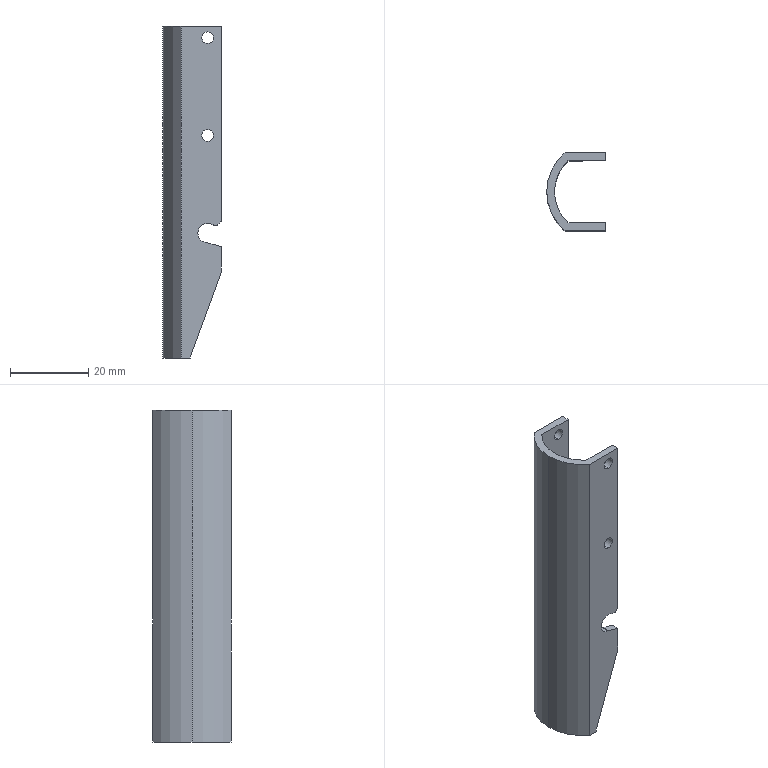Part | SolidWorks | features Fillet 2, ICE 2, Extrusion 1 | 1 solid | 40 faces | box 15 x 20 x 85 mm | volume 6317 mm3 | cylinder 22 | plane 18 | commonest cylinder face diameters 1 x8 3 x8 5 x2 22 x2 26 x2
STEP:
#1=CARTESIAN_POINT('',(-1.5,-8.,83.5));
#2=VERTEX_POINT('',#1);
#3=CARTESIAN_POINT('',(-1.5,-8.,80.5));
#4=VERTEX_POINT('',#3);
#5=CARTESIAN_POINT('',(-1.5,-8.,82.));
#6=DIRECTION('',(0.,-1.,0.));
#7=DIRECTION('',(1.,0.,0.));
#8=AXIS2_PLACEMENT_3D('',#5,#6,#7);
#9=CIRCLE('',#8,1.5);
#10=EDGE_CURVE('',#2,#4,#9,.T.);
#11=ORIENTED_EDGE('',*,*,#10,.F.);
#12=CARTESIAN_POINT('',(-1.5,-10.,83.5));
#13=VERTEX_POINT('',#12);
#14=CARTESIAN_POINT('',(-1.5,10.,83.5));
#15=DIRECTION('',(0.,-1.,0.));
#16=VECTOR('',#15,1000.);
#17=LINE('',#14,#16);
#18=EDGE_CURVE('',#2,#13,#17,.T.);
#19=ORIENTED_EDGE('',*,*,#18,.T.);
#20=CARTESIAN_POINT('',(-1.5,-10.,80.5));
#21=VERTEX_POINT('',#20);
#22=CARTESIAN_POINT('',(-1.5,-10.,82.));
#23=DIRECTION('',(0.,-1.,0.));
#24=DIRECTION('',(0.,0.,-1.));
#25=AXIS2_PLACEMENT_3D('',#22,#23,#24);
#26=CIRCLE('',#25,1.5);
#27=EDGE_CURVE('',#13,#21,#26,.T.);
#28=ORIENTED_EDGE('',*,*,#27,.T.);
#29=CARTESIAN_POINT('',(-1.5,10.,80.5));
#30=DIRECTION('',(0.,-1.,0.));
#31=VECTOR('',#30,1000.);
#32=LINE('',#29,#31);
#33=EDGE_CURVE('',#4,#21,#32,.T.);
#34=ORIENTED_EDGE('',*,*,#33,.F.);
#35=EDGE_LOOP('',(#11,#19,#28,#34));
#36=FACE_OUTER_BOUND('',#35,.T.);
#37=CARTESIAN_POINT('',(-1.5,10.,82.));
#38=DIRECTION('',(0.,-1.,0.));
#39=DIRECTION('',(0.,0.,-1.));
#40=AXIS2_PLACEMENT_3D('',#37,#38,#39);
#41=CYLINDRICAL_SURFACE('',#40,1.5);
#42=ADVANCED_FACE('',(#36),#41,.F.);
#43=CARTESIAN_POINT('',(-1.5,-8.,58.5));
#44=VERTEX_POINT('',#43);
#45=CARTESIAN_POINT('',(-1.5,-8.,55.5));
#46=VERTEX_POINT('',#45);
#47=CARTESIAN_POINT('',(-1.5,-8.,57.));
#48=DIRECTION('',(0.,-1.,0.));
#49=DIRECTION('',(1.,0.,0.));
#50=AXIS2_PLACEMENT_3D('',#47,#48,#49);
#51=CIRCLE('',#50,1.5);
#52=EDGE_CURVE('',#44,#46,#51,.T.);
#53=ORIENTED_EDGE('',*,*,#52,.F.);
#54=CARTESIAN_POINT('',(-1.5,-10.,58.5));
#55=VERTEX_POINT('',#54);
#56=CARTESIAN_POINT('',(-1.5,10.,58.5));
#57=DIRECTION('',(0.,-1.,0.));
#58=VECTOR('',#57,1000.);
#59=LINE('',#56,#58);
#60=EDGE_CURVE('',#44,#55,#59,.T.);
#61=ORIENTED_EDGE('',*,*,#60,.T.);
#62=CARTESIAN_POINT('',(-1.5,-10.,55.5));
#63=VERTEX_POINT('',#62);
#64=CARTESIAN_POINT('',(-1.5,-10.,57.));
#65=DIRECTION('',(0.,-1.,0.));
#66=DIRECTION('',(0.,0.,-1.));
#67=AXIS2_PLACEMENT_3D('',#64,#65,#66);
#68=CIRCLE('',#67,1.5);
#69=EDGE_CURVE('',#55,#63,#68,.T.);
#70=ORIENTED_EDGE('',*,*,#69,.T.);
#71=CARTESIAN_POINT('',(-1.5,10.,55.5));
#72=DIRECTION('',(0.,-1.,0.));
#73=VECTOR('',#72,1000.);
#74=LINE('',#71,#73);
#75=EDGE_CURVE('',#46,#63,#74,.T.);
#76=ORIENTED_EDGE('',*,*,#75,.F.);
#77=EDGE_LOOP('',(#53,#61,#70,#76));
#78=FACE_OUTER_BOUND('',#77,.T.);
#79=CARTESIAN_POINT('',(-1.5,10.,57.));
#80=DIRECTION('',(0.,-1.,0.));
#81=DIRECTION('',(0.,0.,-1.));
#82=AXIS2_PLACEMENT_3D('',#79,#80,#81);
#83=CYLINDRICAL_SURFACE('',#82,1.5);
#84=ADVANCED_FACE('',(#78),#83,.F.);
#85=CARTESIAN_POINT('',(-1.5,10.,83.5));
#86=VERTEX_POINT('',#85);
#87=CARTESIAN_POINT('',(-1.5,10.,80.5));
#88=VERTEX_POINT('',#87);
#89=CARTESIAN_POINT('',(-1.5,10.,82.));
#90=DIRECTION('',(0.,-1.,0.));
#91=DIRECTION('',(0.,0.,-1.));
#92=AXIS2_PLACEMENT_3D('',#89,#90,#91);
#93=CIRCLE('',#92,1.5);
#94=EDGE_CURVE('',#86,#88,#93,.T.);
#95=ORIENTED_EDGE('',*,*,#94,.F.);
#96=CARTESIAN_POINT('',(-1.5,8.,83.5));
#97=VERTEX_POINT('',#96);
#98=CARTESIAN_POINT('',(-1.5,10.,83.5));
#99=DIRECTION('',(0.,-1.,0.));
#100=VECTOR('',#99,1000.);
#101=LINE('',#98,#100);
#102=EDGE_CURVE('',#86,#97,#101,.T.);
#103=ORIENTED_EDGE('',*,*,#102,.T.);
#104=CARTESIAN_POINT('',(-1.5,8.,80.5));
#105=VERTEX_POINT('',#104);
#106=CARTESIAN_POINT('',(-1.5,8.,82.));
#107=DIRECTION('',(0.,1.,0.));
#108=DIRECTION('',(-1.,0.,0.));
#109=AXIS2_PLACEMENT_3D('',#106,#107,#108);
#110=CIRCLE('',#109,1.5);
#111=EDGE_CURVE('',#105,#97,#110,.T.);
#112=ORIENTED_EDGE('',*,*,#111,.F.);
#113=CARTESIAN_POINT('',(-1.5,10.,80.5));
#114=DIRECTION('',(0.,-1.,0.));
#115=VECTOR('',#114,1000.);
#116=LINE('',#113,#115);
#117=EDGE_CURVE('',#88,#105,#116,.T.);
#118=ORIENTED_EDGE('',*,*,#117,.F.);
#119=EDGE_LOOP('',(#95,#103,#112,#118));
#120=FACE_OUTER_BOUND('',#119,.T.);
#121=CARTESIAN_POINT('',(-1.5,10.,82.));
#122=DIRECTION('',(0.,-1.,0.));
#123=DIRECTION('',(0.,0.,-1.));
#124=AXIS2_PLACEMENT_3D('',#121,#122,#123);
#125=CYLINDRICAL_SURFACE('',#124,1.5);
#126=ADVANCED_FACE('',(#120),#125,.F.);
#127=CARTESIAN_POINT('',(-1.5,10.,58.5));
#128=VERTEX_POINT('',#127);
#129=CARTESIAN_POINT('',(-1.5,10.,55.5));
#130=VERTEX_POINT('',#129);
#131=CARTESIAN_POINT('',(-1.5,10.,57.));
#132=DIRECTION('',(0.,-1.,0.));
#133=DIRECTION('',(0.,0.,-1.));
#134=AXIS2_PLACEMENT_3D('',#131,#132,#133);
#135=CIRCLE('',#134,1.5);
#136=EDGE_CURVE('',#128,#130,#135,.T.);
#137=ORIENTED_EDGE('',*,*,#136,.F.);
#138=CARTESIAN_POINT('',(-1.5,8.,58.5));
#139=VERTEX_POINT('',#138);
#140=CARTESIAN_POINT('',(-1.5,10.,58.5));
#141=DIRECTION('',(0.,-1.,0.));
#142=VECTOR('',#141,1000.);
#143=LINE('',#140,#142);
#144=EDGE_CURVE('',#128,#139,#143,.T.);
#145=ORIENTED_EDGE('',*,*,#144,.T.);
#146=CARTESIAN_POINT('',(-1.5,8.,55.5));
#147=VERTEX_POINT('',#146);
#148=CARTESIAN_POINT('',(-1.5,8.,57.));
#149=DIRECTION('',(0.,1.,0.));
#150=DIRECTION('',(-1.,0.,0.));
#151=AXIS2_PLACEMENT_3D('',#148,#149,#150);
#152=CIRCLE('',#151,1.5);
#153=EDGE_CURVE('',#147,#139,#152,.T.);
#154=ORIENTED_EDGE('',*,*,#153,.F.);
#155=CARTESIAN_POINT('',(-1.5,10.,55.5));
#156=DIRECTION('',(0.,-1.,0.));
#157=VECTOR('',#156,1000.);
#158=LINE('',#155,#157);
#159=EDGE_CURVE('',#130,#147,#158,.T.);
#160=ORIENTED_EDGE('',*,*,#159,.F.);
#161=EDGE_LOOP('',(#137,#145,#154,#160));
#162=FACE_OUTER_BOUND('',#161,.T.);
#163=CARTESIAN_POINT('',(-1.5,10.,57.));
#164=DIRECTION('',(0.,-1.,0.));
#165=DIRECTION('',(0.,0.,-1.));
#166=AXIS2_PLACEMENT_3D('',#163,#164,#165);
#167=CYLINDRICAL_SURFACE('',#166,1.5);
#168=ADVANCED_FACE('',(#162),#167,.F.);
#169=CARTESIAN_POINT('',(-11.,0.,85.));
#170=VERTEX_POINT('',#169);
#171=CARTESIAN_POINT('',(-7.55,8.,85.));
#172=VERTEX_POINT('',#171);
#173=CARTESIAN_POINT('',(0.,0.,85.));
#174=DIRECTION('',(0.,0.,-1.));
#175=DIRECTION('',(1.,0.,0.));
#176=AXIS2_PLACEMENT_3D('',#173,#174,#175);
#177=CIRCLE('',#176,11.);
#178=EDGE_CURVE('',#170,#172,#177,.T.);
#179=ORIENTED_EDGE('',*,*,#178,.F.);
#180=CARTESIAN_POINT('',(-11.,0.,0.));
#181=VERTEX_POINT('',#180);
#182=CARTESIAN_POINT('',(-11.,0.,85.));
#183=DIRECTION('',(0.,0.,-1.));
#184=VECTOR('',#183,1000.);
#185=LINE('',#182,#184);
#186=EDGE_CURVE('',#170,#181,#185,.T.);
#187=ORIENTED_EDGE('',*,*,#186,.T.);
#188=CARTESIAN_POINT('',(-7.55,8.,0.));
#189=VERTEX_POINT('',#188);
#190=CARTESIAN_POINT('',(0.,0.,0.));
#191=DIRECTION('',(0.,0.,-1.));
#192=DIRECTION('',(1.,0.,0.));
#193=AXIS2_PLACEMENT_3D('',#190,#191,#192);
#194=CIRCLE('',#193,11.);
#195=EDGE_CURVE('',#181,#189,#194,.T.);
#196=ORIENTED_EDGE('',*,*,#195,.T.);
#197=CARTESIAN_POINT('',(-7.55,8.,85.));
#198=DIRECTION('',(0.,0.,-1.));
#199=VECTOR('',#198,1000.);
#200=LINE('',#197,#199);
#201=EDGE_CURVE('',#172,#189,#200,.T.);
#202=ORIENTED_EDGE('',*,*,#201,.F.);
#203=EDGE_LOOP('',(#179,#187,#196,#202));
#204=FACE_OUTER_BOUND('',#203,.T.);
#205=CARTESIAN_POINT('',(0.,0.,85.));
#206=DIRECTION('',(0.,0.,-1.));
#207=DIRECTION('',(-1.,0.,0.));
#208=AXIS2_PLACEMENT_3D('',#205,#206,#207);
#209=CYLINDRICAL_SURFACE('',#208,11.);
#210=ADVANCED_FACE('',(#204),#209,.F.);
#211=CARTESIAN_POINT('',(-13.,0.,85.));
#212=VERTEX_POINT('',#211);
#213=CARTESIAN_POINT('',(-8.307,-10.,85.));
#214=VERTEX_POINT('',#213);
#215=CARTESIAN_POINT('',(0.,0.,85.));
#216=DIRECTION('',(0.,0.,1.));
#217=DIRECTION('',(1.,0.,0.));
#218=AXIS2_PLACEMENT_3D('',#215,#216,#217);
#219=CIRCLE('',#218,13.);
#220=EDGE_CURVE('',#212,#214,#219,.T.);
#221=ORIENTED_EDGE('',*,*,#220,.F.);
#222=CARTESIAN_POINT('',(-13.,0.,0.));
#223=VERTEX_POINT('',#222);
#224=CARTESIAN_POINT('',(-13.,0.,85.));
#225=DIRECTION('',(0.,0.,-1.));
#226=VECTOR('',#225,1000.);
#227=LINE('',#224,#226);
#228=EDGE_CURVE('',#212,#223,#227,.T.);
#229=ORIENTED_EDGE('',*,*,#228,.T.);
#230=CARTESIAN_POINT('',(-8.307,-10.,0.));
#231=VERTEX_POINT('',#230);
#232=CARTESIAN_POINT('',(0.,0.,0.));
#233=DIRECTION('',(0.,0.,1.));
#234=DIRECTION('',(1.,0.,0.));
#235=AXIS2_PLACEMENT_3D('',#232,#233,#234);
#236=CIRCLE('',#235,13.);
#237=EDGE_CURVE('',#223,#231,#236,.T.);
#238=ORIENTED_EDGE('',*,*,#237,.T.);
#239=CARTESIAN_POINT('',(-8.307,-10.,85.));
#240=DIRECTION('',(0.,0.,-1.));
#241=VECTOR('',#240,1000.);
#242=LINE('',#239,#241);
#243=EDGE_CURVE('',#214,#231,#242,.T.);
#244=ORIENTED_EDGE('',*,*,#243,.F.);
#245=EDGE_LOOP('',(#221,#229,#238,#244));
#246=FACE_OUTER_BOUND('',#245,.T.);
#247=CARTESIAN_POINT('',(0.,0.,85.));
#248=DIRECTION('',(0.,0.,-1.));
#249=DIRECTION('',(-1.,0.,0.));
#250=AXIS2_PLACEMENT_3D('',#247,#248,#249);
#251=CYLINDRICAL_SURFACE('',#250,13.);
#252=ADVANCED_FACE('',(#246),#251,.T.);
#253=CARTESIAN_POINT('',(2.,8.,85.));
#254=VERTEX_POINT('',#253);
#255=CARTESIAN_POINT('',(2.,8.,35.207));
#256=VERTEX_POINT('',#255);
#257=CARTESIAN_POINT('',(2.,8.,85.));
#258=DIRECTION('',(0.,0.,-1.));
#259=VECTOR('',#258,1000.);
#260=LINE('',#257,#259);
#261=EDGE_CURVE('',#254,#256,#260,.T.);
#262=ORIENTED_EDGE('',*,*,#261,.T.);
#263=CARTESIAN_POINT('',(2.,10.,35.207));
#264=VERTEX_POINT('',#263);
#265=CARTESIAN_POINT('',(2.,8.,35.207));
#266=DIRECTION('',(0.,1.,0.));
#267=VECTOR('',#266,1000.);
#268=LINE('',#265,#267);
#269=EDGE_CURVE('',#256,#264,#268,.T.);
#270=ORIENTED_EDGE('',*,*,#269,.T.);
#271=CARTESIAN_POINT('',(2.,10.,85.));
#272=VERTEX_POINT('',#271);
#273=CARTESIAN_POINT('',(2.,10.,85.));
#274=DIRECTION('',(0.,0.,-1.));
#275=VECTOR('',#274,1000.);
#276=LINE('',#273,#275);
#277=EDGE_CURVE('',#272,#264,#276,.T.);
#278=ORIENTED_EDGE('',*,*,#277,.F.);
#279=CARTESIAN_POINT('',(2.,8.,85.));
#280=DIRECTION('',(0.,1.,0.));
#281=VECTOR('',#280,1000.);
#282=LINE('',#279,#281);
#283=EDGE_CURVE('',#254,#272,#282,.T.);
#284=ORIENTED_EDGE('',*,*,#283,.F.);
#285=EDGE_LOOP('',(#262,#270,#278,#284));
#286=FACE_OUTER_BOUND('',#285,.T.);
#287=CARTESIAN_POINT('',(2.,8.,85.));
#288=DIRECTION('',(-1.,0.,0.));
#289=DIRECTION('',(0.,0.,1.));
#290=AXIS2_PLACEMENT_3D('',#287,#288,#289);
#291=PLANE('',#290);
#292=ADVANCED_FACE('',(#286),#291,.F.);
#293=CARTESIAN_POINT('',(2.,-10.,85.));
#294=VERTEX_POINT('',#293);
#295=CARTESIAN_POINT('',(2.,-10.,35.207));
#296=VERTEX_POINT('',#295);
#297=CARTESIAN_POINT('',(2.,-10.,85.));
#298=DIRECTION('',(0.,0.,-1.));
#299=VECTOR('',#298,1000.);
#300=LINE('',#297,#299);
#301=EDGE_CURVE('',#294,#296,#300,.T.);
#302=ORIENTED_EDGE('',*,*,#301,.T.);
#303=CARTESIAN_POINT('',(2.,-8.,35.207));
#304=VERTEX_POINT('',#303);
#305=CARTESIAN_POINT('',(2.,-8.,35.207));
#306=DIRECTION('',(0.,1.,0.));
#307=VECTOR('',#306,1000.);
#308=LINE('',#305,#307);
#309=EDGE_CURVE('',#296,#304,#308,.T.);
#310=ORIENTED_EDGE('',*,*,#309,.T.);
#311=CARTESIAN_POINT('',(2.,-8.,85.));
#312=VERTEX_POINT('',#311);
#313=CARTESIAN_POINT('',(2.,-8.,85.));
#314=DIRECTION('',(0.,0.,-1.));
#315=VECTOR('',#314,1000.);
#316=LINE('',#313,#315);
#317=EDGE_CURVE('',#312,#304,#316,.T.);
#318=ORIENTED_EDGE('',*,*,#317,.F.);
#319=CARTESIAN_POINT('',(2.,-8.,85.));
#320=DIRECTION('',(0.,1.,0.));
#321=VECTOR('',#320,1000.);
#322=LINE('',#319,#321);
#323=EDGE_CURVE('',#294,#312,#322,.T.);
#324=ORIENTED_EDGE('',*,*,#323,.F.);
#325=EDGE_LOOP('',(#302,#310,#318,#324));
#326=FACE_OUTER_BOUND('',#325,.T.);
#327=CARTESIAN_POINT('',(2.,-8.,85.));
#328=DIRECTION('',(-1.,0.,0.));
#329=DIRECTION('',(0.,0.,1.));
#330=AXIS2_PLACEMENT_3D('',#327,#328,#329);
#331=PLANE('',#330);
#332=ADVANCED_FACE('',(#326),#331,.F.);
#333=CARTESIAN_POINT('',(2.,10.,28.5));
#334=VERTEX_POINT('',#333);
#335=CARTESIAN_POINT('',(2.,10.,22.));
#336=VERTEX_POINT('',#335);
#337=CARTESIAN_POINT('',(2.,10.,85.));
#338=DIRECTION('',(0.,0.,-1.));
#339=VECTOR('',#338,1000.);
#340=LINE('',#337,#339);
#341=EDGE_CURVE('',#334,#336,#340,.T.);
#342=ORIENTED_EDGE('',*,*,#341,.F.);
#343=CARTESIAN_POINT('',(2.,8.,28.5));
#344=VERTEX_POINT('',#343);
#345=CARTESIAN_POINT('',(2.,10.,28.5));
#346=DIRECTION('',(0.,-1.,0.));
#347=VECTOR('',#346,1000.);
#348=LINE('',#345,#347);
#349=EDGE_CURVE('',#334,#344,#348,.T.);
#350=ORIENTED_EDGE('',*,*,#349,.T.);
#351=CARTESIAN_POINT('',(2.,8.,22.));
#352=VERTEX_POINT('',#351);
#353=CARTESIAN_POINT('',(2.,8.,85.));
#354=DIRECTION('',(0.,0.,-1.));
#355=VECTOR('',#354,1000.);
#356=LINE('',#353,#355);
#357=EDGE_CURVE('',#344,#352,#356,.T.);
#358=ORIENTED_EDGE('',*,*,#357,.T.);
#359=CARTESIAN_POINT('',(2.,10.,22.));
#360=DIRECTION('',(0.,-1.,0.));
#361=VECTOR('',#360,1000.);
#362=LINE('',#359,#361);
#363=EDGE_CURVE('',#336,#352,#362,.T.);
#364=ORIENTED_EDGE('',*,*,#363,.F.);
#365=EDGE_LOOP('',(#342,#350,#358,#364));
#366=FACE_OUTER_BOUND('',#365,.T.);
#367=CARTESIAN_POINT('',(2.,8.,85.));
#368=DIRECTION('',(-1.,0.,0.));
#369=DIRECTION('',(0.,0.,1.));
#370=AXIS2_PLACEMENT_3D('',#367,#368,#369);
#371=PLANE('',#370);
#372=ADVANCED_FACE('',(#366),#371,.F.);
#373=CARTESIAN_POINT('',(-0.1181,10.,34.083));
#374=VERTEX_POINT('',#373);
#375=CARTESIAN_POINT('',(-1.561,10.,29.501));
#376=VERTEX_POINT('',#375);
#377=CARTESIAN_POINT('',(-1.5,10.,32.));
#378=DIRECTION('',(0.,-1.,0.));
#379=DIRECTION('',(1.,0.,0.));
#380=AXIS2_PLACEMENT_3D('',#377,#378,#379);
#381=CIRCLE('',#380,2.5);
#382=EDGE_CURVE('',#374,#376,#381,.T.);
#383=ORIENTED_EDGE('',*,*,#382,.T.);
#384=CARTESIAN_POINT('',(-1.436,10.,29.482));
#385=VERTEX_POINT('',#384);
#386=CARTESIAN_POINT('',(-1.573,10.,29.001));
#387=DIRECTION('',(0.,1.,0.));
#388=DIRECTION('',(1.,0.,0.));
#389=AXIS2_PLACEMENT_3D('',#386,#387,#388);
#390=CIRCLE('',#389,0.5);
#391=EDGE_CURVE('',#376,#385,#390,.T.);
#392=ORIENTED_EDGE('',*,*,#391,.T.);
#393=CARTESIAN_POINT('',(-1.5,10.,29.5));
#394=DIRECTION('',(0.9615,0.,-0.2747));
#395=VECTOR('',#394,1000.);
#396=LINE('',#393,#395);
#397=EDGE_CURVE('',#385,#334,#396,.T.);
#398=ORIENTED_EDGE('',*,*,#397,.T.);
#399=ORIENTED_EDGE('',*,*,#341,.T.);
#400=CARTESIAN_POINT('',(-6.,10.,0.));
#401=VERTEX_POINT('',#400);
#402=CARTESIAN_POINT('',(2.,10.,22.));
#403=DIRECTION('',(-0.3417,0.,-0.9398));
#404=VECTOR('',#403,1000.);
#405=LINE('',#402,#404);
#406=EDGE_CURVE('',#336,#401,#405,.T.);
#407=ORIENTED_EDGE('',*,*,#406,.T.);
#408=CARTESIAN_POINT('',(-8.307,10.,0.));
#409=VERTEX_POINT('',#408);
#410=CARTESIAN_POINT('',(-8.307,10.,0.));
#411=DIRECTION('',(-1.,0.,0.));
#412=VECTOR('',#411,1000.);
#413=LINE('',#410,#412);
#414=EDGE_CURVE('',#401,#409,#413,.T.);
#415=ORIENTED_EDGE('',*,*,#414,.T.);
#416=CARTESIAN_POINT('',(-8.307,10.,85.));
#417=VERTEX_POINT('',#416);
#418=CARTESIAN_POINT('',(-8.307,10.,85.));
#419=DIRECTION('',(0.,0.,-1.));
#420=VECTOR('',#419,1000.);
#421=LINE('',#418,#420);
#422=EDGE_CURVE('',#417,#409,#421,.T.);
#423=ORIENTED_EDGE('',*,*,#422,.F.);
#424=CARTESIAN_POINT('',(-8.307,10.,85.));
#425=DIRECTION('',(-1.,0.,0.));
#426=VECTOR('',#425,1000.);
#427=LINE('',#424,#426);
#428=EDGE_CURVE('',#272,#417,#427,.T.);
#429=ORIENTED_EDGE('',*,*,#428,.F.);
#430=ORIENTED_EDGE('',*,*,#277,.T.);
#431=CARTESIAN_POINT('',(1.854,10.,34.854));
#432=VERTEX_POINT('',#431);
#433=CARTESIAN_POINT('',(1.5,10.,35.207));
#434=DIRECTION('',(0.,1.,0.));
#435=DIRECTION('',(1.,0.,0.));
#436=AXIS2_PLACEMENT_3D('',#433,#434,#435);
#437=CIRCLE('',#436,0.5);
#438=EDGE_CURVE('',#264,#432,#437,.T.);
#439=ORIENTED_EDGE('',*,*,#438,.T.);
#440=CARTESIAN_POINT('',(1.146,10.,34.146));
#441=VERTEX_POINT('',#440);
#442=CARTESIAN_POINT('',(1.,10.,34.));
#443=DIRECTION('',(-0.7071,0.,-0.7071));
#444=VECTOR('',#443,1000.);
#445=LINE('',#442,#444);
#446=EDGE_CURVE('',#432,#441,#445,.T.);
#447=ORIENTED_EDGE('',*,*,#446,.T.);
#448=CARTESIAN_POINT('',(0.7929,10.,34.));
#449=VERTEX_POINT('',#448);
#450=CARTESIAN_POINT('',(0.7929,10.,34.5));
#451=DIRECTION('',(0.,1.,0.));
#452=DIRECTION('',(1.,0.,0.));
#453=AXIS2_PLACEMENT_3D('',#450,#451,#452);
#454=CIRCLE('',#453,0.5);
#455=EDGE_CURVE('',#441,#449,#454,.T.);
#456=ORIENTED_EDGE('',*,*,#455,.T.);
#457=CARTESIAN_POINT('',(0.1583,10.,34.));
#458=VERTEX_POINT('',#457);
#459=CARTESIAN_POINT('',(0.,10.,34.));
#460=DIRECTION('',(-1.,0.,0.));
#461=VECTOR('',#460,1000.);
#462=LINE('',#459,#461);
#463=EDGE_CURVE('',#449,#458,#462,.T.);
#464=ORIENTED_EDGE('',*,*,#463,.T.);
#465=CARTESIAN_POINT('',(0.1583,10.,34.5));
#466=DIRECTION('',(0.,1.,0.));
#467=DIRECTION('',(1.,0.,0.));
#468=AXIS2_PLACEMENT_3D('',#465,#466,#467);
#469=CIRCLE('',#468,0.5);
#470=EDGE_CURVE('',#458,#374,#469,.T.);
#471=ORIENTED_EDGE('',*,*,#470,.T.);
#472=EDGE_LOOP('',(#383,#392,#398,#399,#407,#415,#423,#429,#430,#439,#447,#456,#464,#471));
#473=FACE_OUTER_BOUND('',#472,.T.);
#474=CARTESIAN_POINT('',(-1.5,10.,82.));
#475=DIRECTION('',(0.,-1.,0.));
#476=DIRECTION('',(0.,0.,-1.));
#477=AXIS2_PLACEMENT_3D('',#474,#475,#476);
#478=CIRCLE('',#477,1.5);
#479=EDGE_CURVE('',#88,#86,#478,.T.);
#480=ORIENTED_EDGE('',*,*,#479,.T.);
#481=ORIENTED_EDGE('',*,*,#94,.T.);
#482=EDGE_LOOP('',(#480,#481));
#483=FACE_BOUND('',#482,.T.);
#484=CARTESIAN_POINT('',(-1.5,10.,57.));
#485=DIRECTION('',(0.,-1.,0.));
#486=DIRECTION('',(0.,0.,-1.));
#487=AXIS2_PLACEMENT_3D('',#484,#485,#486);
#488=CIRCLE('',#487,1.5);
#489=EDGE_CURVE('',#130,#128,#488,.T.);
#490=ORIENTED_EDGE('',*,*,#489,.T.);
#491=ORIENTED_EDGE('',*,*,#136,.T.);
#492=EDGE_LOOP('',(#490,#491));
#493=FACE_BOUND('',#492,.T.);
#494=CARTESIAN_POINT('',(-8.307,10.,85.));
#495=DIRECTION('',(0.,-1.,0.));
#496=DIRECTION('',(1.,0.,0.));
#497=AXIS2_PLACEMENT_3D('',#494,#495,#496);
#498=PLANE('',#497);
#499=ADVANCED_FACE('',(#473,#483,#493),#498,.F.);
#500=ORIENTED_EDGE('',*,*,#228,.F.);
#501=CARTESIAN_POINT('',(0.,0.,85.));
#502=DIRECTION('',(0.,0.,1.));
#503=DIRECTION('',(1.,0.,0.));
#504=AXIS2_PLACEMENT_3D('',#501,#502,#503);
#505=CIRCLE('',#504,13.);
#506=EDGE_CURVE('',#417,#212,#505,.T.);
#507=ORIENTED_EDGE('',*,*,#506,.F.);
#508=ORIENTED_EDGE('',*,*,#422,.T.);
#509=CARTESIAN_POINT('',(0.,0.,0.));
#510=DIRECTION('',(0.,0.,1.));
#511=DIRECTION('',(1.,0.,0.));
#512=AXIS2_PLACEMENT_3D('',#509,#510,#511);
#513=CIRCLE('',#512,13.);
#514=EDGE_CURVE('',#409,#223,#513,.T.);
#515=ORIENTED_EDGE('',*,*,#514,.T.);
#516=EDGE_LOOP('',(#500,#507,#508,#515));
#517=FACE_OUTER_BOUND('',#516,.T.);
#518=CARTESIAN_POINT('',(0.,0.,85.));
#519=DIRECTION('',(0.,0.,-1.));
#520=DIRECTION('',(-1.,0.,0.));
#521=AXIS2_PLACEMENT_3D('',#518,#519,#520);
#522=CYLINDRICAL_SURFACE('',#521,13.);
#523=ADVANCED_FACE('',(#517),#522,.T.);
#524=CARTESIAN_POINT('',(-1.5,-10.,82.));
#525=DIRECTION('',(0.,-1.,0.));
#526=DIRECTION('',(0.,0.,-1.));
#527=AXIS2_PLACEMENT_3D('',#524,#525,#526);
#528=CIRCLE('',#527,1.5);
#529=EDGE_CURVE('',#21,#13,#528,.T.);
#530=ORIENTED_EDGE('',*,*,#529,.F.);
#531=ORIENTED_EDGE('',*,*,#27,.F.);
#532=EDGE_LOOP('',(#530,#531));
#533=FACE_BOUND('',#532,.T.);
#534=CARTESIAN_POINT('',(-1.5,-10.,57.));
#535=DIRECTION('',(0.,-1.,0.));
#536=DIRECTION('',(0.,0.,-1.));
#537=AXIS2_PLACEMENT_3D('',#534,#535,#536);
#538=CIRCLE('',#537,1.5);
#539=EDGE_CURVE('',#63,#55,#538,.T.);
#540=ORIENTED_EDGE('',*,*,#539,.F.);
#541=ORIENTED_EDGE('',*,*,#69,.F.);
#542=EDGE_LOOP('',(#540,#541));
#543=FACE_BOUND('',#542,.T.);
#544=CARTESIAN_POINT('',(-1.436,-10.,29.482));
#545=VERTEX_POINT('',#544);
#546=CARTESIAN_POINT('',(2.,-10.,28.5));
#547=VERTEX_POINT('',#546);
#548=CARTESIAN_POINT('',(-1.5,-10.,29.5));
#549=DIRECTION('',(0.9615,0.,-0.2747));
#550=VECTOR('',#549,1000.);
#551=LINE('',#548,#550);
#552=EDGE_CURVE('',#545,#547,#551,.T.);
#553=ORIENTED_EDGE('',*,*,#552,.F.);
#554=CARTESIAN_POINT('',(-1.561,-10.,29.501));
#555=VERTEX_POINT('',#554);
#556=CARTESIAN_POINT('',(-1.573,-10.,29.001));
#557=DIRECTION('',(0.,-1.,0.));
#558=DIRECTION('',(-1.,0.,0.));
#559=AXIS2_PLACEMENT_3D('',#556,#557,#558);
#560=CIRCLE('',#559,0.5);
#561=EDGE_CURVE('',#545,#555,#560,.T.);
#562=ORIENTED_EDGE('',*,*,#561,.T.);
#563=CARTESIAN_POINT('',(-0.1181,-10.,34.083));
#564=VERTEX_POINT('',#563);
#565=CARTESIAN_POINT('',(-1.5,-10.,32.));
#566=DIRECTION('',(0.,-1.,0.));
#567=DIRECTION('',(1.,0.,0.));
#568=AXIS2_PLACEMENT_3D('',#565,#566,#567);
#569=CIRCLE('',#568,2.5);
#570=EDGE_CURVE('',#564,#555,#569,.T.);
#571=ORIENTED_EDGE('',*,*,#570,.F.);
#572=CARTESIAN_POINT('',(0.1583,-10.,34.));
#573=VERTEX_POINT('',#572);
#574=CARTESIAN_POINT('',(0.1583,-10.,34.5));
#575=DIRECTION('',(0.,-1.,0.));
#576=DIRECTION('',(-1.,0.,0.));
#577=AXIS2_PLACEMENT_3D('',#574,#575,#576);
#578=CIRCLE('',#577,0.5);
#579=EDGE_CURVE('',#564,#573,#578,.T.);
#580=ORIENTED_EDGE('',*,*,#579,.T.);
#581=CARTESIAN_POINT('',(0.7929,-10.,34.));
#582=VERTEX_POINT('',#581);
#583=CARTESIAN_POINT('',(0.,-10.,34.));
#584=DIRECTION('',(-1.,0.,0.));
#585=VECTOR('',#584,1000.);
#586=LINE('',#583,#585);
#587=EDGE_CURVE('',#582,#573,#586,.T.);
#588=ORIENTED_EDGE('',*,*,#587,.F.);
#589=CARTESIAN_POINT('',(1.146,-10.,34.146));
#590=VERTEX_POINT('',#589);
#591=CARTESIAN_POINT('',(0.7929,-10.,34.5));
#592=DIRECTION('',(0.,-1.,0.));
#593=DIRECTION('',(-1.,0.,0.));
#594=AXIS2_PLACEMENT_3D('',#591,#592,#593);
#595=CIRCLE('',#594,0.5);
#596=EDGE_CURVE('',#582,#590,#595,.T.);
#597=ORIENTED_EDGE('',*,*,#596,.T.);
#598=CARTESIAN_POINT('',(1.854,-10.,34.854));
#599=VERTEX_POINT('',#598);
#600=CARTESIAN_POINT('',(1.,-10.,34.));
#601=DIRECTION('',(-0.7071,0.,-0.7071));
#602=VECTOR('',#601,1000.);
#603=LINE('',#600,#602);
#604=EDGE_CURVE('',#599,#590,#603,.T.);
#605=ORIENTED_EDGE('',*,*,#604,.F.);
#606=CARTESIAN_POINT('',(1.5,-10.,35.207));
#607=DIRECTION('',(0.,-1.,0.));
#608=DIRECTION('',(-1.,0.,0.));
#609=AXIS2_PLACEMENT_3D('',#606,#607,#608);
#610=CIRCLE('',#609,0.5);
#611=EDGE_CURVE('',#599,#296,#610,.T.);
#612=ORIENTED_EDGE('',*,*,#611,.T.);
#613=ORIENTED_EDGE('',*,*,#301,.F.);
#614=CARTESIAN_POINT('',(-8.307,-10.,85.));
#615=DIRECTION('',(1.,0.,0.));
#616=VECTOR('',#615,1000.);
#617=LINE('',#614,#616);
#618=EDGE_CURVE('',#214,#294,#617,.T.);
#619=ORIENTED_EDGE('',*,*,#618,.F.);
#620=ORIENTED_EDGE('',*,*,#243,.T.);
#621=CARTESIAN_POINT('',(-6.,-10.,0.));
#622=VERTEX_POINT('',#621);
#623=CARTESIAN_POINT('',(-8.307,-10.,0.));
#624=DIRECTION('',(1.,0.,0.));
#625=VECTOR('',#624,1000.);
#626=LINE('',#623,#625);
#627=EDGE_CURVE('',#231,#622,#626,.T.);
#628=ORIENTED_EDGE('',*,*,#627,.T.);
#629=CARTESIAN_POINT('',(2.,-10.,22.));
#630=VERTEX_POINT('',#629);
#631=CARTESIAN_POINT('',(2.,-10.,22.));
#632=DIRECTION('',(-0.3417,0.,-0.9398));
#633=VECTOR('',#632,1000.);
#634=LINE('',#631,#633);
#635=EDGE_CURVE('',#630,#622,#634,.T.);
#636=ORIENTED_EDGE('',*,*,#635,.F.);
#637=CARTESIAN_POINT('',(2.,-10.,85.));
#638=DIRECTION('',(0.,0.,-1.));
#639=VECTOR('',#638,1000.);
#640=LINE('',#637,#639);
#641=EDGE_CURVE('',#547,#630,#640,.T.);
#642=ORIENTED_EDGE('',*,*,#641,.F.);
#643=EDGE_LOOP('',(#553,#562,#571,#580,#588,#597,#605,#612,#613,#619,#620,#628,#636,#642));
#644=FACE_OUTER_BOUND('',#643,.T.);
#645=CARTESIAN_POINT('',(-8.307,-10.,85.));
#646=DIRECTION('',(0.,1.,0.));
#647=DIRECTION('',(-1.,0.,0.));
#648=AXIS2_PLACEMENT_3D('',#645,#646,#647);
#649=PLANE('',#648);
#650=ADVANCED_FACE('',(#533,#543,#644),#649,.F.);
#651=CARTESIAN_POINT('',(2.,-8.,28.5));
#652=VERTEX_POINT('',#651);
#653=CARTESIAN_POINT('',(2.,-8.,22.));
#654=VERTEX_POINT('',#653);
#655=CARTESIAN_POINT('',(2.,-8.,85.));
#656=DIRECTION('',(0.,0.,-1.));
#657=VECTOR('',#656,1000.);
#658=LINE('',#655,#657);
#659=EDGE_CURVE('',#652,#654,#658,.T.);
#660=ORIENTED_EDGE('',*,*,#659,.F.);
#661=CARTESIAN_POINT('',(2.,10.,28.5));
#662=DIRECTION('',(0.,-1.,0.));
#663=VECTOR('',#662,1000.);
#664=LINE('',#661,#663);
#665=EDGE_CURVE('',#652,#547,#664,.T.);
#666=ORIENTED_EDGE('',*,*,#665,.T.);
#667=ORIENTED_EDGE('',*,*,#641,.T.);
#668=CARTESIAN_POINT('',(2.,10.,22.));
#669=DIRECTION('',(0.,-1.,0.));
#670=VECTOR('',#669,1000.);
#671=LINE('',#668,#670);
#672=EDGE_CURVE('',#654,#630,#671,.T.);
#673=ORIENTED_EDGE('',*,*,#672,.F.);
#674=EDGE_LOOP('',(#660,#666,#667,#673));
#675=FACE_OUTER_BOUND('',#674,.T.);
#676=CARTESIAN_POINT('',(2.,-8.,85.));
#677=DIRECTION('',(-1.,0.,0.));
#678=DIRECTION('',(0.,0.,1.));
#679=AXIS2_PLACEMENT_3D('',#676,#677,#678);
#680=PLANE('',#679);
#681=ADVANCED_FACE('',(#675),#680,.F.);
#682=CARTESIAN_POINT('',(-0.1181,-8.,34.083));
#683=VERTEX_POINT('',#682);
#684=CARTESIAN_POINT('',(-1.561,-8.,29.501));
#685=VERTEX_POINT('',#684);
#686=CARTESIAN_POINT('',(-1.5,-8.,32.));
#687=DIRECTION('',(0.,-1.,0.));
#688=DIRECTION('',(1.,0.,0.));
#689=AXIS2_PLACEMENT_3D('',#686,#687,#688);
#690=CIRCLE('',#689,2.5);
#691=EDGE_CURVE('',#683,#685,#690,.T.);
#692=ORIENTED_EDGE('',*,*,#691,.T.);
#693=CARTESIAN_POINT('',(-1.436,-8.,29.482));
#694=VERTEX_POINT('',#693);
#695=CARTESIAN_POINT('',(-1.573,-8.,29.001));
#696=DIRECTION('',(0.,1.,0.));
#697=DIRECTION('',(1.,0.,0.));
#698=AXIS2_PLACEMENT_3D('',#695,#696,#697);
#699=CIRCLE('',#698,0.5);
#700=EDGE_CURVE('',#685,#694,#699,.T.);
#701=ORIENTED_EDGE('',*,*,#700,.T.);
#702=CARTESIAN_POINT('',(-21.754,-8.,35.287));
#703=DIRECTION('',(0.9615,0.,-0.2747));
#704=VECTOR('',#703,1000.);
#705=LINE('',#702,#704);
#706=EDGE_CURVE('',#694,#652,#705,.T.);
#707=ORIENTED_EDGE('',*,*,#706,.T.);
#708=ORIENTED_EDGE('',*,*,#659,.T.);
#709=CARTESIAN_POINT('',(-6.,-8.,0.));
#710=VERTEX_POINT('',#709);
#711=CARTESIAN_POINT('',(21.118,-8.,74.575));
#712=DIRECTION('',(-0.3417,0.,-0.9398));
#713=VECTOR('',#712,1000.);
#714=LINE('',#711,#713);
#715=EDGE_CURVE('',#654,#710,#714,.T.);
#716=ORIENTED_EDGE('',*,*,#715,.T.);
#717=CARTESIAN_POINT('',(-7.55,-8.,0.));
#718=VERTEX_POINT('',#717);
#719=CARTESIAN_POINT('',(-7.55,-8.,0.));
#720=DIRECTION('',(-1.,0.,0.));
#721=VECTOR('',#720,1000.);
#722=LINE('',#719,#721);
#723=EDGE_CURVE('',#710,#718,#722,.T.);
#724=ORIENTED_EDGE('',*,*,#723,.T.);
#725=CARTESIAN_POINT('',(-7.55,-8.,85.));
#726=VERTEX_POINT('',#725);
#727=CARTESIAN_POINT('',(-7.55,-8.,85.));
#728=DIRECTION('',(0.,0.,-1.));
#729=VECTOR('',#728,1000.);
#730=LINE('',#727,#729);
#731=EDGE_CURVE('',#726,#718,#730,.T.);
#732=ORIENTED_EDGE('',*,*,#731,.F.);
#733=CARTESIAN_POINT('',(-7.55,-8.,85.));
#734=DIRECTION('',(-1.,0.,0.));
#735=VECTOR('',#734,1000.);
#736=LINE('',#733,#735);
#737=EDGE_CURVE('',#312,#726,#736,.T.);
#738=ORIENTED_EDGE('',*,*,#737,.F.);
#739=ORIENTED_EDGE('',*,*,#317,.T.);
#740=CARTESIAN_POINT('',(1.854,-8.,34.854));
#741=VERTEX_POINT('',#740);
#742=CARTESIAN_POINT('',(1.5,-8.,35.207));
#743=DIRECTION('',(0.,1.,0.));
#744=DIRECTION('',(1.,0.,0.));
#745=AXIS2_PLACEMENT_3D('',#742,#743,#744);
#746=CIRCLE('',#745,0.5);
#747=EDGE_CURVE('',#304,#741,#746,.T.);
#748=ORIENTED_EDGE('',*,*,#747,.T.);
#749=CARTESIAN_POINT('',(1.146,-8.,34.146));
#750=VERTEX_POINT('',#749);
#751=CARTESIAN_POINT('',(22.225,-8.,55.225));
#752=DIRECTION('',(-0.7071,0.,-0.7071));
#753=VECTOR('',#752,1000.);
#754=LINE('',#751,#753);
#755=EDGE_CURVE('',#741,#750,#754,.T.);
#756=ORIENTED_EDGE('',*,*,#755,.T.);
#757=CARTESIAN_POINT('',(0.7929,-8.,34.));
#758=VERTEX_POINT('',#757);
#759=CARTESIAN_POINT('',(0.7929,-8.,34.5));
#760=DIRECTION('',(0.,1.,0.));
#761=DIRECTION('',(1.,0.,0.));
#762=AXIS2_PLACEMENT_3D('',#759,#760,#761);
#763=CIRCLE('',#762,0.5);
#764=EDGE_CURVE('',#750,#758,#763,.T.);
#765=ORIENTED_EDGE('',*,*,#764,.T.);
#766=CARTESIAN_POINT('',(0.1583,-8.,34.));
#767=VERTEX_POINT('',#766);
#768=CARTESIAN_POINT('',(-7.55,-8.,34.));
#769=DIRECTION('',(-1.,0.,0.));
#770=VECTOR('',#769,1000.);
#771=LINE('',#768,#770);
#772=EDGE_CURVE('',#758,#767,#771,.T.);
#773=ORIENTED_EDGE('',*,*,#772,.T.);
#774=CARTESIAN_POINT('',(0.1583,-8.,34.5));
#775=DIRECTION('',(0.,1.,0.));
#776=DIRECTION('',(1.,0.,0.));
#777=AXIS2_PLACEMENT_3D('',#774,#775,#776);
#778=CIRCLE('',#777,0.5);
#779=EDGE_CURVE('',#767,#683,#778,.T.);
#780=ORIENTED_EDGE('',*,*,#779,.T.);
#781=EDGE_LOOP('',(#692,#701,#707,#708,#716,#724,#732,#738,#739,#748,#756,#765,#773,#780));
#782=FACE_OUTER_BOUND('',#781,.T.);
#783=CARTESIAN_POINT('',(-1.5,-8.,82.));
#784=DIRECTION('',(0.,-1.,0.));
#785=DIRECTION('',(1.,0.,0.));
#786=AXIS2_PLACEMENT_3D('',#783,#784,#785);
#787=CIRCLE('',#786,1.5);
#788=EDGE_CURVE('',#4,#2,#787,.T.);
#789=ORIENTED_EDGE('',*,*,#788,.T.);
#790=ORIENTED_EDGE('',*,*,#10,.T.);
#791=EDGE_LOOP('',(#789,#790));
#792=FACE_BOUND('',#791,.T.);
#793=CARTESIAN_POINT('',(-1.5,-8.,57.));
#794=DIRECTION('',(0.,-1.,0.));
#795=DIRECTION('',(1.,0.,0.));
#796=AXIS2_PLACEMENT_3D('',#793,#794,#795);
#797=CIRCLE('',#796,1.5);
#798=EDGE_CURVE('',#46,#44,#797,.T.);
#799=ORIENTED_EDGE('',*,*,#798,.T.);
#800=ORIENTED_EDGE('',*,*,#52,.T.);
#801=EDGE_LOOP('',(#799,#800));
#802=FACE_BOUND('',#801,.T.);
#803=CARTESIAN_POINT('',(-7.55,-8.,85.));
#804=DIRECTION('',(0.,-1.,0.));
#805=DIRECTION('',(1.,0.,0.));
#806=AXIS2_PLACEMENT_3D('',#803,#804,#805);
#807=PLANE('',#806);
#808=ADVANCED_FACE('',(#782,#792,#802),#807,.F.);
#809=ORIENTED_EDGE('',*,*,#186,.F.);
#810=CARTESIAN_POINT('',(0.,0.,85.));
#811=DIRECTION('',(0.,0.,-1.));
#812=DIRECTION('',(1.,0.,0.));
#813=AXIS2_PLACEMENT_3D('',#810,#811,#812);
#814=CIRCLE('',#813,11.);
#815=EDGE_CURVE('',#726,#170,#814,.T.);
#816=ORIENTED_EDGE('',*,*,#815,.F.);
#817=ORIENTED_EDGE('',*,*,#731,.T.);
#818=CARTESIAN_POINT('',(0.,0.,0.));
#819=DIRECTION('',(0.,0.,-1.));
#820=DIRECTION('',(1.,0.,0.));
#821=AXIS2_PLACEMENT_3D('',#818,#819,#820);
#822=CIRCLE('',#821,11.);
#823=EDGE_CURVE('',#718,#181,#822,.T.);
#824=ORIENTED_EDGE('',*,*,#823,.T.);
#825=EDGE_LOOP('',(#809,#816,#817,#824));
#826=FACE_OUTER_BOUND('',#825,.T.);
#827=CARTESIAN_POINT('',(0.,0.,85.));
#828=DIRECTION('',(0.,0.,-1.));
#829=DIRECTION('',(-1.,0.,0.));
#830=AXIS2_PLACEMENT_3D('',#827,#828,#829);
#831=CYLINDRICAL_SURFACE('',#830,11.);
#832=ADVANCED_FACE('',(#826),#831,.F.);
#833=ORIENTED_EDGE('',*,*,#111,.T.);
#834=CARTESIAN_POINT('',(-1.5,8.,82.));
#835=DIRECTION('',(0.,1.,0.));
#836=DIRECTION('',(-1.,0.,0.));
#837=AXIS2_PLACEMENT_3D('',#834,#835,#836);
#838=CIRCLE('',#837,1.5);
#839=EDGE_CURVE('',#97,#105,#838,.T.);
#840=ORIENTED_EDGE('',*,*,#839,.T.);
#841=EDGE_LOOP('',(#833,#840));
#842=FACE_BOUND('',#841,.T.);
#843=ORIENTED_EDGE('',*,*,#153,.T.);
#844=CARTESIAN_POINT('',(-1.5,8.,57.));
#845=DIRECTION('',(0.,1.,0.));
#846=DIRECTION('',(-1.,0.,0.));
#847=AXIS2_PLACEMENT_3D('',#844,#845,#846);
#848=CIRCLE('',#847,1.5);
#849=EDGE_CURVE('',#139,#147,#848,.T.);
#850=ORIENTED_EDGE('',*,*,#849,.T.);
#851=EDGE_LOOP('',(#843,#850));
#852=FACE_BOUND('',#851,.T.);
#853=CARTESIAN_POINT('',(-1.436,8.,29.482));
#854=VERTEX_POINT('',#853);
#855=CARTESIAN_POINT('',(-21.754,8.,35.287));
#856=DIRECTION('',(-0.9615,0.,0.2747));
#857=VECTOR('',#856,1000.);
#858=LINE('',#855,#857);
#859=EDGE_CURVE('',#344,#854,#858,.T.);
#860=ORIENTED_EDGE('',*,*,#859,.T.);
#861=CARTESIAN_POINT('',(-1.561,8.,29.501));
#862=VERTEX_POINT('',#861);
#863=CARTESIAN_POINT('',(-1.573,8.,29.001));
#864=DIRECTION('',(0.,-1.,0.));
#865=DIRECTION('',(-1.,0.,0.));
#866=AXIS2_PLACEMENT_3D('',#863,#864,#865);
#867=CIRCLE('',#866,0.5);
#868=EDGE_CURVE('',#854,#862,#867,.T.);
#869=ORIENTED_EDGE('',*,*,#868,.T.);
#870=CARTESIAN_POINT('',(-0.1181,8.,34.083));
#871=VERTEX_POINT('',#870);
#872=CARTESIAN_POINT('',(-1.5,8.,32.));
#873=DIRECTION('',(0.,1.,0.));
#874=DIRECTION('',(-1.,0.,0.));
#875=AXIS2_PLACEMENT_3D('',#872,#873,#874);
#876=CIRCLE('',#875,2.5);
#877=EDGE_CURVE('',#862,#871,#876,.T.);
#878=ORIENTED_EDGE('',*,*,#877,.T.);
#879=CARTESIAN_POINT('',(0.1583,8.,34.));
#880=VERTEX_POINT('',#879);
#881=CARTESIAN_POINT('',(0.1583,8.,34.5));
#882=DIRECTION('',(0.,-1.,0.));
#883=DIRECTION('',(-1.,0.,0.));
#884=AXIS2_PLACEMENT_3D('',#881,#882,#883);
#885=CIRCLE('',#884,0.5);
#886=EDGE_CURVE('',#871,#880,#885,.T.);
#887=ORIENTED_EDGE('',*,*,#886,.T.);
#888=CARTESIAN_POINT('',(0.7929,8.,34.));
#889=VERTEX_POINT('',#888);
#890=CARTESIAN_POINT('',(-7.55,8.,34.));
#891=DIRECTION('',(1.,0.,0.));
#892=VECTOR('',#891,1000.);
#893=LINE('',#890,#892);
#894=EDGE_CURVE('',#880,#889,#893,.T.);
#895=ORIENTED_EDGE('',*,*,#894,.T.);
#896=CARTESIAN_POINT('',(1.146,8.,34.146));
#897=VERTEX_POINT('',#896);
#898=CARTESIAN_POINT('',(0.7929,8.,34.5));
#899=DIRECTION('',(0.,-1.,0.));
#900=DIRECTION('',(-1.,0.,0.));
#901=AXIS2_PLACEMENT_3D('',#898,#899,#900);
#902=CIRCLE('',#901,0.5);
#903=EDGE_CURVE('',#889,#897,#902,.T.);
#904=ORIENTED_EDGE('',*,*,#903,.T.);
#905=CARTESIAN_POINT('',(1.854,8.,34.854));
#906=VERTEX_POINT('',#905);
#907=CARTESIAN_POINT('',(22.225,8.,55.225));
#908=DIRECTION('',(0.7071,0.,0.7071));
#909=VECTOR('',#908,1000.);
#910=LINE('',#907,#909);
#911=EDGE_CURVE('',#897,#906,#910,.T.);
#912=ORIENTED_EDGE('',*,*,#911,.T.);
#913=CARTESIAN_POINT('',(1.5,8.,35.207));
#914=DIRECTION('',(0.,-1.,0.));
#915=DIRECTION('',(-1.,0.,0.));
#916=AXIS2_PLACEMENT_3D('',#913,#914,#915);
#917=CIRCLE('',#916,0.5);
#918=EDGE_CURVE('',#906,#256,#917,.T.);
#919=ORIENTED_EDGE('',*,*,#918,.T.);
#920=ORIENTED_EDGE('',*,*,#261,.F.);
#921=CARTESIAN_POINT('',(-7.55,8.,85.));
#922=DIRECTION('',(1.,0.,0.));
#923=VECTOR('',#922,1000.);
#924=LINE('',#921,#923);
#925=EDGE_CURVE('',#172,#254,#924,.T.);
#926=ORIENTED_EDGE('',*,*,#925,.F.);
#927=ORIENTED_EDGE('',*,*,#201,.T.);
#928=CARTESIAN_POINT('',(-6.,8.,0.));
#929=VERTEX_POINT('',#928);
#930=CARTESIAN_POINT('',(-7.55,8.,0.));
#931=DIRECTION('',(1.,0.,0.));
#932=VECTOR('',#931,1000.);
#933=LINE('',#930,#932);
#934=EDGE_CURVE('',#189,#929,#933,.T.);
#935=ORIENTED_EDGE('',*,*,#934,.T.);
#936=CARTESIAN_POINT('',(21.118,8.,74.575));
#937=DIRECTION('',(0.3417,0.,0.9398));
#938=VECTOR('',#937,1000.);
#939=LINE('',#936,#938);
#940=EDGE_CURVE('',#929,#352,#939,.T.);
#941=ORIENTED_EDGE('',*,*,#940,.T.);
#942=ORIENTED_EDGE('',*,*,#357,.F.);
#943=EDGE_LOOP('',(#860,#869,#878,#887,#895,#904,#912,#919,#920,#926,#927,#935,#941,#942));
#944=FACE_OUTER_BOUND('',#943,.T.);
#945=CARTESIAN_POINT('',(-7.55,8.,85.));
#946=DIRECTION('',(0.,1.,0.));
#947=DIRECTION('',(-1.,0.,0.));
#948=AXIS2_PLACEMENT_3D('',#945,#946,#947);
#949=PLANE('',#948);
#950=ADVANCED_FACE('',(#842,#852,#944),#949,.F.);
#951=ORIENTED_EDGE('',*,*,#283,.T.);
#952=ORIENTED_EDGE('',*,*,#428,.T.);
#953=ORIENTED_EDGE('',*,*,#506,.T.);
#954=ORIENTED_EDGE('',*,*,#220,.T.);
#955=ORIENTED_EDGE('',*,*,#618,.T.);
#956=ORIENTED_EDGE('',*,*,#323,.T.);
#957=ORIENTED_EDGE('',*,*,#737,.T.);
#958=ORIENTED_EDGE('',*,*,#815,.T.);
#959=ORIENTED_EDGE('',*,*,#178,.T.);
#960=ORIENTED_EDGE('',*,*,#925,.T.);
#961=EDGE_LOOP('',(#951,#952,#953,#954,#955,#956,#957,#958,#959,#960));
#962=FACE_OUTER_BOUND('',#961,.T.);
#963=CARTESIAN_POINT('',(0.,0.,85.));
#964=DIRECTION('',(0.,0.,1.));
#965=DIRECTION('',(1.,0.,0.));
#966=AXIS2_PLACEMENT_3D('',#963,#964,#965);
#967=PLANE('',#966);
#968=ADVANCED_FACE('',(#962),#967,.T.);
#969=ORIENTED_EDGE('',*,*,#414,.F.);
#970=CARTESIAN_POINT('',(-6.,10.,0.));
#971=DIRECTION('',(0.,-1.,0.));
#972=VECTOR('',#971,1000.);
#973=LINE('',#970,#972);
#974=EDGE_CURVE('',#401,#929,#973,.T.);
#975=ORIENTED_EDGE('',*,*,#974,.T.);
#976=ORIENTED_EDGE('',*,*,#934,.F.);
#977=ORIENTED_EDGE('',*,*,#195,.F.);
#978=ORIENTED_EDGE('',*,*,#823,.F.);
#979=ORIENTED_EDGE('',*,*,#723,.F.);
#980=CARTESIAN_POINT('',(-6.,0.,0.));
#981=DIRECTION('',(0.,-1.,0.));
#982=VECTOR('',#981,1000.);
#983=LINE('',#980,#982);
#984=EDGE_CURVE('',#710,#622,#983,.T.);
#985=ORIENTED_EDGE('',*,*,#984,.T.);
#986=ORIENTED_EDGE('',*,*,#627,.F.);
#987=ORIENTED_EDGE('',*,*,#237,.F.);
#988=ORIENTED_EDGE('',*,*,#514,.F.);
#989=EDGE_LOOP('',(#969,#975,#976,#977,#978,#979,#985,#986,#987,#988));
#990=FACE_OUTER_BOUND('',#989,.T.);
#991=CARTESIAN_POINT('',(0.,0.,0.));
#992=DIRECTION('',(0.,0.,1.));
#993=DIRECTION('',(1.,0.,0.));
#994=AXIS2_PLACEMENT_3D('',#991,#992,#993);
#995=PLANE('',#994);
#996=ADVANCED_FACE('',(#990),#995,.F.);
#997=ORIENTED_EDGE('',*,*,#672,.T.);
#998=ORIENTED_EDGE('',*,*,#635,.T.);
#999=ORIENTED_EDGE('',*,*,#984,.F.);
#1000=ORIENTED_EDGE('',*,*,#715,.F.);
#1001=EDGE_LOOP('',(#997,#998,#999,#1000));
#1002=FACE_OUTER_BOUND('',#1001,.T.);
#1003=CARTESIAN_POINT('',(2.,10.,22.));
#1004=DIRECTION('',(-0.9398,0.,0.3417));
#1005=DIRECTION('',(0.3417,0.,0.9398));
#1006=AXIS2_PLACEMENT_3D('',#1003,#1004,#1005);
#1007=PLANE('',#1006);
#1008=ADVANCED_FACE('',(#1002),#1007,.F.);
#1009=ORIENTED_EDGE('',*,*,#974,.F.);
#1010=ORIENTED_EDGE('',*,*,#406,.F.);
#1011=ORIENTED_EDGE('',*,*,#363,.T.);
#1012=ORIENTED_EDGE('',*,*,#940,.F.);
#1013=EDGE_LOOP('',(#1009,#1010,#1011,#1012));
#1014=FACE_OUTER_BOUND('',#1013,.T.);
#1015=CARTESIAN_POINT('',(2.,10.,22.));
#1016=DIRECTION('',(-0.9398,0.,0.3417));
#1017=DIRECTION('',(0.3417,0.,0.9398));
#1018=AXIS2_PLACEMENT_3D('',#1015,#1016,#1017);
#1019=PLANE('',#1018);
#1020=ADVANCED_FACE('',(#1014),#1019,.F.);
#1021=ORIENTED_EDGE('',*,*,#144,.F.);
#1022=ORIENTED_EDGE('',*,*,#489,.F.);
#1023=ORIENTED_EDGE('',*,*,#159,.T.);
#1024=ORIENTED_EDGE('',*,*,#849,.F.);
#1025=EDGE_LOOP('',(#1021,#1022,#1023,#1024));
#1026=FACE_OUTER_BOUND('',#1025,.T.);
#1027=CARTESIAN_POINT('',(-1.5,10.,57.));
#1028=DIRECTION('',(0.,-1.,0.));
#1029=DIRECTION('',(0.,0.,-1.));
#1030=AXIS2_PLACEMENT_3D('',#1027,#1028,#1029);
#1031=CYLINDRICAL_SURFACE('',#1030,1.5);
#1032=ADVANCED_FACE('',(#1026),#1031,.F.);
#1033=ORIENTED_EDGE('',*,*,#102,.F.);
#1034=ORIENTED_EDGE('',*,*,#479,.F.);
#1035=ORIENTED_EDGE('',*,*,#117,.T.);
#1036=ORIENTED_EDGE('',*,*,#839,.F.);
#1037=EDGE_LOOP('',(#1033,#1034,#1035,#1036));
#1038=FACE_OUTER_BOUND('',#1037,.T.);
#1039=CARTESIAN_POINT('',(-1.5,10.,82.));
#1040=DIRECTION('',(0.,-1.,0.));
#1041=DIRECTION('',(0.,0.,-1.));
#1042=AXIS2_PLACEMENT_3D('',#1039,#1040,#1041);
#1043=CYLINDRICAL_SURFACE('',#1042,1.5);
#1044=ADVANCED_FACE('',(#1038),#1043,.F.);
#1045=ORIENTED_EDGE('',*,*,#60,.F.);
#1046=ORIENTED_EDGE('',*,*,#798,.F.);
#1047=ORIENTED_EDGE('',*,*,#75,.T.);
#1048=ORIENTED_EDGE('',*,*,#539,.T.);
#1049=EDGE_LOOP('',(#1045,#1046,#1047,#1048));
#1050=FACE_OUTER_BOUND('',#1049,.T.);
#1051=CARTESIAN_POINT('',(-1.5,10.,57.));
#1052=DIRECTION('',(0.,-1.,0.));
#1053=DIRECTION('',(0.,0.,-1.));
#1054=AXIS2_PLACEMENT_3D('',#1051,#1052,#1053);
#1055=CYLINDRICAL_SURFACE('',#1054,1.5);
#1056=ADVANCED_FACE('',(#1050),#1055,.F.);
#1057=ORIENTED_EDGE('',*,*,#18,.F.);
#1058=ORIENTED_EDGE('',*,*,#788,.F.);
#1059=ORIENTED_EDGE('',*,*,#33,.T.);
#1060=ORIENTED_EDGE('',*,*,#529,.T.);
#1061=EDGE_LOOP('',(#1057,#1058,#1059,#1060));
#1062=FACE_OUTER_BOUND('',#1061,.T.);
#1063=CARTESIAN_POINT('',(-1.5,10.,82.));
#1064=DIRECTION('',(0.,-1.,0.));
#1065=DIRECTION('',(0.,0.,-1.));
#1066=AXIS2_PLACEMENT_3D('',#1063,#1064,#1065);
#1067=CYLINDRICAL_SURFACE('',#1066,1.5);
#1068=ADVANCED_FACE('',(#1062),#1067,.F.);
#1069=ORIENTED_EDGE('',*,*,#463,.F.);
#1070=CARTESIAN_POINT('',(0.7929,10.,34.));
#1071=DIRECTION('',(0.,-1.,0.));
#1072=VECTOR('',#1071,1000.);
#1073=LINE('',#1070,#1072);
#1074=EDGE_CURVE('',#449,#889,#1073,.T.);
#1075=ORIENTED_EDGE('',*,*,#1074,.T.);
#1076=ORIENTED_EDGE('',*,*,#894,.F.);
#1077=CARTESIAN_POINT('',(0.1583,10.,34.));
#1078=DIRECTION('',(0.,1.,0.));
#1079=VECTOR('',#1078,1000.);
#1080=LINE('',#1077,#1079);
#1081=EDGE_CURVE('',#880,#458,#1080,.T.);
#1082=ORIENTED_EDGE('',*,*,#1081,.T.);
#1083=EDGE_LOOP('',(#1069,#1075,#1076,#1082));
#1084=FACE_OUTER_BOUND('',#1083,.T.);
#1085=CARTESIAN_POINT('',(0.,10.,34.));
#1086=DIRECTION('',(0.,0.,1.));
#1087=DIRECTION('',(1.,0.,0.));
#1088=AXIS2_PLACEMENT_3D('',#1085,#1086,#1087);
#1089=PLANE('',#1088);
#1090=ADVANCED_FACE('',(#1084),#1089,.F.);
#1091=ORIENTED_EDGE('',*,*,#877,.F.);
#1092=CARTESIAN_POINT('',(-1.561,10.,29.501));
#1093=DIRECTION('',(0.,1.,0.));
#1094=VECTOR('',#1093,1000.);
#1095=LINE('',#1092,#1094);
#1096=EDGE_CURVE('',#862,#376,#1095,.T.);
#1097=ORIENTED_EDGE('',*,*,#1096,.T.);
#1098=ORIENTED_EDGE('',*,*,#382,.F.);
#1099=CARTESIAN_POINT('',(-0.1181,10.,34.083));
#1100=DIRECTION('',(0.,-1.,0.));
#1101=VECTOR('',#1100,1000.);
#1102=LINE('',#1099,#1101);
#1103=EDGE_CURVE('',#374,#871,#1102,.T.);
#1104=ORIENTED_EDGE('',*,*,#1103,.T.);
#1105=EDGE_LOOP('',(#1091,#1097,#1098,#1104));
#1106=FACE_OUTER_BOUND('',#1105,.T.);
#1107=CARTESIAN_POINT('',(-1.5,10.,32.));
#1108=DIRECTION('',(0.,-1.,0.));
#1109=DIRECTION('',(1.,0.,0.));
#1110=AXIS2_PLACEMENT_3D('',#1107,#1108,#1109);
#1111=CYLINDRICAL_SURFACE('',#1110,2.5);
#1112=ADVANCED_FACE('',(#1106),#1111,.F.);
#1113=ORIENTED_EDGE('',*,*,#397,.F.);
#1114=CARTESIAN_POINT('',(-1.436,10.,29.482));
#1115=DIRECTION('',(0.,-1.,0.));
#1116=VECTOR('',#1115,1000.);
#1117=LINE('',#1114,#1116);
#1118=EDGE_CURVE('',#385,#854,#1117,.T.);
#1119=ORIENTED_EDGE('',*,*,#1118,.T.);
#1120=ORIENTED_EDGE('',*,*,#859,.F.);
#1121=ORIENTED_EDGE('',*,*,#349,.F.);
#1122=EDGE_LOOP('',(#1113,#1119,#1120,#1121));
#1123=FACE_OUTER_BOUND('',#1122,.T.);
#1124=CARTESIAN_POINT('',(-1.5,10.,29.5));
#1125=DIRECTION('',(-0.2747,0.,-0.9615));
#1126=DIRECTION('',(-0.9615,0.,0.2747));
#1127=AXIS2_PLACEMENT_3D('',#1124,#1125,#1126);
#1128=PLANE('',#1127);
#1129=ADVANCED_FACE('',(#1123),#1128,.F.);
#1130=ORIENTED_EDGE('',*,*,#911,.F.);
#1131=CARTESIAN_POINT('',(1.146,10.,34.146));
#1132=DIRECTION('',(0.,1.,0.));
#1133=VECTOR('',#1132,1000.);
#1134=LINE('',#1131,#1133);
#1135=EDGE_CURVE('',#897,#441,#1134,.T.);
#1136=ORIENTED_EDGE('',*,*,#1135,.T.);
#1137=ORIENTED_EDGE('',*,*,#446,.F.);
#1138=CARTESIAN_POINT('',(1.854,10.,34.854));
#1139=DIRECTION('',(0.,-1.,0.));
#1140=VECTOR('',#1139,1000.);
#1141=LINE('',#1138,#1140);
#1142=EDGE_CURVE('',#432,#906,#1141,.T.);
#1143=ORIENTED_EDGE('',*,*,#1142,.T.);
#1144=EDGE_LOOP('',(#1130,#1136,#1137,#1143));
#1145=FACE_OUTER_BOUND('',#1144,.T.);
#1146=CARTESIAN_POINT('',(1.,10.,34.));
#1147=DIRECTION('',(-0.7071,0.,0.7071));
#1148=DIRECTION('',(0.7071,0.,0.7071));
#1149=AXIS2_PLACEMENT_3D('',#1146,#1147,#1148);
#1150=PLANE('',#1149);
#1151=ADVANCED_FACE('',(#1145),#1150,.F.);
#1152=ORIENTED_EDGE('',*,*,#755,.F.);
#1153=CARTESIAN_POINT('',(1.854,10.,34.854));
#1154=DIRECTION('',(0.,-1.,0.));
#1155=VECTOR('',#1154,1000.);
#1156=LINE('',#1153,#1155);
#1157=EDGE_CURVE('',#741,#599,#1156,.T.);
#1158=ORIENTED_EDGE('',*,*,#1157,.T.);
#1159=ORIENTED_EDGE('',*,*,#604,.T.);
#1160=CARTESIAN_POINT('',(1.146,10.,34.146));
#1161=DIRECTION('',(0.,1.,0.));
#1162=VECTOR('',#1161,1000.);
#1163=LINE('',#1160,#1162);
#1164=EDGE_CURVE('',#590,#750,#1163,.T.);
#1165=ORIENTED_EDGE('',*,*,#1164,.T.);
#1166=EDGE_LOOP('',(#1152,#1158,#1159,#1165));
#1167=FACE_OUTER_BOUND('',#1166,.T.);
#1168=CARTESIAN_POINT('',(1.,10.,34.));
#1169=DIRECTION('',(-0.7071,0.,0.7071));
#1170=DIRECTION('',(0.7071,0.,0.7071));
#1171=AXIS2_PLACEMENT_3D('',#1168,#1169,#1170);
#1172=PLANE('',#1171);
#1173=ADVANCED_FACE('',(#1167),#1172,.F.);
#1174=ORIENTED_EDGE('',*,*,#706,.F.);
#1175=CARTESIAN_POINT('',(-1.436,10.,29.482));
#1176=DIRECTION('',(0.,-1.,0.));
#1177=VECTOR('',#1176,1000.);
#1178=LINE('',#1175,#1177);
#1179=EDGE_CURVE('',#694,#545,#1178,.T.);
#1180=ORIENTED_EDGE('',*,*,#1179,.T.);
#1181=ORIENTED_EDGE('',*,*,#552,.T.);
#1182=ORIENTED_EDGE('',*,*,#665,.F.);
#1183=EDGE_LOOP('',(#1174,#1180,#1181,#1182));
#1184=FACE_OUTER_BOUND('',#1183,.T.);
#1185=CARTESIAN_POINT('',(-1.5,10.,29.5));
#1186=DIRECTION('',(-0.2747,0.,-0.9615));
#1187=DIRECTION('',(-0.9615,0.,0.2747));
#1188=AXIS2_PLACEMENT_3D('',#1185,#1186,#1187);
#1189=PLANE('',#1188);
#1190=ADVANCED_FACE('',(#1184),#1189,.F.);
#1191=ORIENTED_EDGE('',*,*,#570,.T.);
#1192=CARTESIAN_POINT('',(-1.561,10.,29.501));
#1193=DIRECTION('',(0.,1.,0.));
#1194=VECTOR('',#1193,1000.);
#1195=LINE('',#1192,#1194);
#1196=EDGE_CURVE('',#555,#685,#1195,.T.);
#1197=ORIENTED_EDGE('',*,*,#1196,.T.);
#1198=ORIENTED_EDGE('',*,*,#691,.F.);
#1199=CARTESIAN_POINT('',(-0.1181,10.,34.083));
#1200=DIRECTION('',(0.,-1.,0.));
#1201=VECTOR('',#1200,1000.);
#1202=LINE('',#1199,#1201);
#1203=EDGE_CURVE('',#683,#564,#1202,.T.);
#1204=ORIENTED_EDGE('',*,*,#1203,.T.);
#1205=EDGE_LOOP('',(#1191,#1197,#1198,#1204));
#1206=FACE_OUTER_BOUND('',#1205,.T.);
#1207=CARTESIAN_POINT('',(-1.5,10.,32.));
#1208=DIRECTION('',(0.,-1.,0.));
#1209=DIRECTION('',(1.,0.,0.));
#1210=AXIS2_PLACEMENT_3D('',#1207,#1208,#1209);
#1211=CYLINDRICAL_SURFACE('',#1210,2.5);
#1212=ADVANCED_FACE('',(#1206),#1211,.F.);
#1213=ORIENTED_EDGE('',*,*,#772,.F.);
#1214=CARTESIAN_POINT('',(0.7929,10.,34.));
#1215=DIRECTION('',(0.,-1.,0.));
#1216=VECTOR('',#1215,1000.);
#1217=LINE('',#1214,#1216);
#1218=EDGE_CURVE('',#758,#582,#1217,.T.);
#1219=ORIENTED_EDGE('',*,*,#1218,.T.);
#1220=ORIENTED_EDGE('',*,*,#587,.T.);
#1221=CARTESIAN_POINT('',(0.1583,10.,34.));
#1222=DIRECTION('',(0.,1.,0.));
#1223=VECTOR('',#1222,1000.);
#1224=LINE('',#1221,#1223);
#1225=EDGE_CURVE('',#573,#767,#1224,.T.);
#1226=ORIENTED_EDGE('',*,*,#1225,.T.);
#1227=EDGE_LOOP('',(#1213,#1219,#1220,#1226));
#1228=FACE_OUTER_BOUND('',#1227,.T.);
#1229=CARTESIAN_POINT('',(0.,10.,34.));
#1230=DIRECTION('',(0.,0.,1.));
#1231=DIRECTION('',(1.,0.,0.));
#1232=AXIS2_PLACEMENT_3D('',#1229,#1230,#1231);
#1233=PLANE('',#1232);
#1234=ADVANCED_FACE('',(#1228),#1233,.F.);
#1235=ORIENTED_EDGE('',*,*,#747,.F.);
#1236=ORIENTED_EDGE('',*,*,#309,.F.);
#1237=ORIENTED_EDGE('',*,*,#611,.F.);
#1238=ORIENTED_EDGE('',*,*,#1157,.F.);
#1239=EDGE_LOOP('',(#1235,#1236,#1237,#1238));
#1240=FACE_OUTER_BOUND('',#1239,.T.);
#1241=CARTESIAN_POINT('',(1.5,10.,35.207));
#1242=DIRECTION('',(0.,-1.,0.));
#1243=DIRECTION('',(0.,0.,-1.));
#1244=AXIS2_PLACEMENT_3D('',#1241,#1242,#1243);
#1245=CYLINDRICAL_SURFACE('',#1244,0.5);
#1246=ADVANCED_FACE('',(#1240),#1245,.T.);
#1247=ORIENTED_EDGE('',*,*,#764,.F.);
#1248=ORIENTED_EDGE('',*,*,#1164,.F.);
#1249=ORIENTED_EDGE('',*,*,#596,.F.);
#1250=ORIENTED_EDGE('',*,*,#1218,.F.);
#1251=EDGE_LOOP('',(#1247,#1248,#1249,#1250));
#1252=FACE_OUTER_BOUND('',#1251,.T.);
#1253=CARTESIAN_POINT('',(0.7929,10.,34.5));
#1254=DIRECTION('',(0.,-1.,0.));
#1255=DIRECTION('',(1.,0.,0.));
#1256=AXIS2_PLACEMENT_3D('',#1253,#1254,#1255);
#1257=CYLINDRICAL_SURFACE('',#1256,0.5);
#1258=ADVANCED_FACE('',(#1252),#1257,.T.);
#1259=ORIENTED_EDGE('',*,*,#455,.F.);
#1260=ORIENTED_EDGE('',*,*,#1135,.F.);
#1261=ORIENTED_EDGE('',*,*,#903,.F.);
#1262=ORIENTED_EDGE('',*,*,#1074,.F.);
#1263=EDGE_LOOP('',(#1259,#1260,#1261,#1262));
#1264=FACE_OUTER_BOUND('',#1263,.T.);
#1265=CARTESIAN_POINT('',(0.7929,10.,34.5));
#1266=DIRECTION('',(0.,-1.,0.));
#1267=DIRECTION('',(1.,0.,0.));
#1268=AXIS2_PLACEMENT_3D('',#1265,#1266,#1267);
#1269=CYLINDRICAL_SURFACE('',#1268,0.5);
#1270=ADVANCED_FACE('',(#1264),#1269,.T.);
#1271=ORIENTED_EDGE('',*,*,#438,.F.);
#1272=ORIENTED_EDGE('',*,*,#269,.F.);
#1273=ORIENTED_EDGE('',*,*,#918,.F.);
#1274=ORIENTED_EDGE('',*,*,#1142,.F.);
#1275=EDGE_LOOP('',(#1271,#1272,#1273,#1274));
#1276=FACE_OUTER_BOUND('',#1275,.T.);
#1277=CARTESIAN_POINT('',(1.5,10.,35.207));
#1278=DIRECTION('',(0.,-1.,0.));
#1279=DIRECTION('',(0.,0.,-1.));
#1280=AXIS2_PLACEMENT_3D('',#1277,#1278,#1279);
#1281=CYLINDRICAL_SURFACE('',#1280,0.5);
#1282=ADVANCED_FACE('',(#1276),#1281,.T.);
#1283=ORIENTED_EDGE('',*,*,#779,.F.);
#1284=ORIENTED_EDGE('',*,*,#1225,.F.);
#1285=ORIENTED_EDGE('',*,*,#579,.F.);
#1286=ORIENTED_EDGE('',*,*,#1203,.F.);
#1287=EDGE_LOOP('',(#1283,#1284,#1285,#1286));
#1288=FACE_OUTER_BOUND('',#1287,.T.);
#1289=CARTESIAN_POINT('',(0.1583,10.,34.5));
#1290=DIRECTION('',(0.,-1.,0.));
#1291=DIRECTION('',(1.,0.,0.));
#1292=AXIS2_PLACEMENT_3D('',#1289,#1290,#1291);
#1293=CYLINDRICAL_SURFACE('',#1292,0.5);
#1294=ADVANCED_FACE('',(#1288),#1293,.T.);
#1295=ORIENTED_EDGE('',*,*,#470,.F.);
#1296=ORIENTED_EDGE('',*,*,#1081,.F.);
#1297=ORIENTED_EDGE('',*,*,#886,.F.);
#1298=ORIENTED_EDGE('',*,*,#1103,.F.);
#1299=EDGE_LOOP('',(#1295,#1296,#1297,#1298));
#1300=FACE_OUTER_BOUND('',#1299,.T.);
#1301=CARTESIAN_POINT('',(0.1583,10.,34.5));
#1302=DIRECTION('',(0.,-1.,0.));
#1303=DIRECTION('',(1.,0.,0.));
#1304=AXIS2_PLACEMENT_3D('',#1301,#1302,#1303);
#1305=CYLINDRICAL_SURFACE('',#1304,0.5);
#1306=ADVANCED_FACE('',(#1300),#1305,.T.);
#1307=ORIENTED_EDGE('',*,*,#391,.F.);
#1308=ORIENTED_EDGE('',*,*,#1096,.F.);
#1309=ORIENTED_EDGE('',*,*,#868,.F.);
#1310=ORIENTED_EDGE('',*,*,#1118,.F.);
#1311=EDGE_LOOP('',(#1307,#1308,#1309,#1310));
#1312=FACE_OUTER_BOUND('',#1311,.T.);
#1313=CARTESIAN_POINT('',(-1.573,10.,29.001));
#1314=DIRECTION('',(0.,-1.,0.));
#1315=DIRECTION('',(1.,0.,0.));
#1316=AXIS2_PLACEMENT_3D('',#1313,#1314,#1315);
#1317=CYLINDRICAL_SURFACE('',#1316,0.5);
#1318=ADVANCED_FACE('',(#1312),#1317,.T.);
#1319=ORIENTED_EDGE('',*,*,#700,.F.);
#1320=ORIENTED_EDGE('',*,*,#1196,.F.);
#1321=ORIENTED_EDGE('',*,*,#561,.F.);
#1322=ORIENTED_EDGE('',*,*,#1179,.F.);
#1323=EDGE_LOOP('',(#1319,#1320,#1321,#1322));
#1324=FACE_OUTER_BOUND('',#1323,.T.);
#1325=CARTESIAN_POINT('',(-1.573,10.,29.001));
#1326=DIRECTION('',(0.,-1.,0.));
#1327=DIRECTION('',(1.,0.,0.));
#1328=AXIS2_PLACEMENT_3D('',#1325,#1326,#1327);
#1329=CYLINDRICAL_SURFACE('',#1328,0.5);
#1330=ADVANCED_FACE('',(#1324),#1329,.T.);
#1331=CLOSED_SHELL('',(#42,#84,#126,#168,#210,#252,#292,#332,#372,#499,#523,#650,#681,#808,#832,#950,#968,#996,#1008,#1020,#1032,#1044,#1056,#1068,#1090,#1112,#1129,#1151,#1173,#1190,#1212,#1234,#1246,#1258,#1270,#1282,#1294,#1306,#1318,#1330));
#1332=MANIFOLD_SOLID_BREP('',#1331);
#1333=CARTESIAN_POINT('',(0.,0.,0.));
#1334=DIRECTION('',(0.,0.,1.));
#1335=DIRECTION('',(1.,0.,0.));
#1336=AXIS2_PLACEMENT_3D('',#1333,#1334,#1335);
#1337=(LENGTH_UNIT()NAMED_UNIT(*)SI_UNIT(.MILLI.,.METRE.));
#1338=UNCERTAINTY_MEASURE_WITH_UNIT(LENGTH_MEASURE(0.00001),#1337,'','');
#1339=(NAMED_UNIT(*)PLANE_ANGLE_UNIT()SI_UNIT($,.RADIAN.));
#1340=(NAMED_UNIT(*)SI_UNIT($,.STERADIAN.)SOLID_ANGLE_UNIT());
#1341=(GEOMETRIC_REPRESENTATION_CONTEXT(3)GLOBAL_UNCERTAINTY_ASSIGNED_CONTEXT((#1338))GLOBAL_UNIT_ASSIGNED_CONTEXT((#1337,#1339,#1340))REPRESENTATION_CONTEXT('',''));
#1342=ADVANCED_BREP_SHAPE_REPRESENTATION('',(#1332,#1336),#1341);